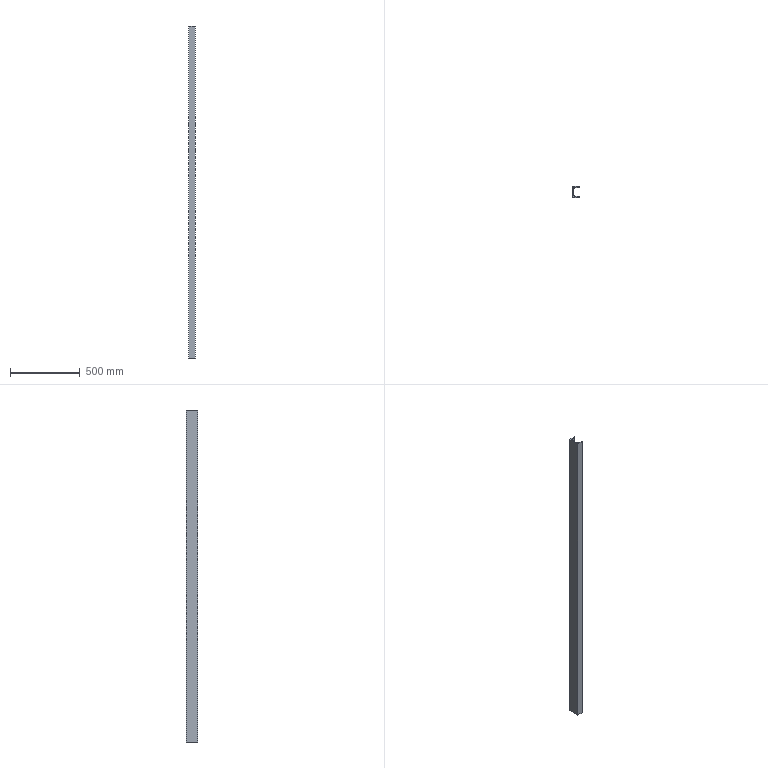Part | STEP file | 750038140 | 1 solid | 14 faces | box 43 x 80 x 2374 mm | volume 2431604 mm3 | plane 10 | cylinder 4 | commonest cylinder face diameters 8 x2 16 x2
STEP:
#1=CARTESIAN_POINT('',(0.,0.,2374.));
#2=VERTEX_POINT('',#1);
#3=CARTESIAN_POINT('',(0.,0.,0.));
#4=VERTEX_POINT('',#3);
#5=CARTESIAN_POINT('',(0.,0.,2374.));
#6=DIRECTION('',(0.,0.,-1.));
#7=VECTOR('',#6,1000.);
#8=LINE('',#5,#7);
#9=EDGE_CURVE('',#2,#4,#8,.T.);
#10=ORIENTED_EDGE('',*,*,#9,.F.);
#11=CARTESIAN_POINT('',(0.,80.,2374.));
#12=VERTEX_POINT('',#11);
#13=CARTESIAN_POINT('',(0.,80.,2374.));
#14=DIRECTION('',(0.,-1.,0.));
#15=VECTOR('',#14,1000.);
#16=LINE('',#13,#15);
#17=EDGE_CURVE('',#12,#2,#16,.T.);
#18=ORIENTED_EDGE('',*,*,#17,.F.);
#19=CARTESIAN_POINT('',(0.,80.,0.));
#20=VERTEX_POINT('',#19);
#21=CARTESIAN_POINT('',(0.,80.,2374.));
#22=DIRECTION('',(0.,0.,1.));
#23=VECTOR('',#22,1000.);
#24=LINE('',#21,#23);
#25=EDGE_CURVE('',#20,#12,#24,.T.);
#26=ORIENTED_EDGE('',*,*,#25,.F.);
#27=CARTESIAN_POINT('',(0.,80.,0.));
#28=DIRECTION('',(0.,1.,0.));
#29=VECTOR('',#28,1000.);
#30=LINE('',#27,#29);
#31=EDGE_CURVE('',#4,#20,#30,.T.);
#32=ORIENTED_EDGE('',*,*,#31,.F.);
#33=EDGE_LOOP('',(#10,#18,#26,#32));
#34=FACE_OUTER_BOUND('',#33,.T.);
#35=CARTESIAN_POINT('',(0.,80.,2374.));
#36=DIRECTION('',(1.,0.,0.));
#37=DIRECTION('',(0.,0.,-1.));
#38=AXIS2_PLACEMENT_3D('',#35,#36,#37);
#39=PLANE('',#38);
#40=ADVANCED_FACE('',(#34),#39,.F.);
#41=CARTESIAN_POINT('',(43.,80.,0.));
#42=VERTEX_POINT('',#41);
#43=CARTESIAN_POINT('',(39.,80.,0.));
#44=DIRECTION('',(-1.,0.,0.));
#45=VECTOR('',#44,1000.);
#46=LINE('',#43,#45);
#47=EDGE_CURVE('',#42,#20,#46,.T.);
#48=ORIENTED_EDGE('',*,*,#47,.F.);
#49=CARTESIAN_POINT('',(43.,77.52,0.));
#50=VERTEX_POINT('',#49);
#51=CARTESIAN_POINT('',(43.,2.48,0.));
#52=DIRECTION('',(0.,1.,0.));
#53=VECTOR('',#52,1000.);
#54=LINE('',#51,#53);
#55=EDGE_CURVE('',#50,#42,#54,.T.);
#56=ORIENTED_EDGE('',*,*,#55,.F.);
#57=CARTESIAN_POINT('',(39.398,73.54,0.));
#58=VERTEX_POINT('',#57);
#59=CARTESIAN_POINT('',(39.,77.52,0.));
#60=DIRECTION('',(0.,0.,1.));
#61=DIRECTION('',(-1.,0.,0.));
#62=AXIS2_PLACEMENT_3D('',#59,#60,#61);
#63=CIRCLE('',#62,4.);
#64=EDGE_CURVE('',#58,#50,#63,.T.);
#65=ORIENTED_EDGE('',*,*,#64,.F.);
#66=CARTESIAN_POINT('',(12.204,70.82,0.));
#67=VERTEX_POINT('',#66);
#68=CARTESIAN_POINT('',(12.204,70.82,0.));
#69=DIRECTION('',(0.995,0.0995,0.));
#70=VECTOR('',#69,1000.);
#71=LINE('',#68,#70);
#72=EDGE_CURVE('',#67,#58,#71,.T.);
#73=ORIENTED_EDGE('',*,*,#72,.F.);
#74=CARTESIAN_POINT('',(5.,62.86,0.));
#75=VERTEX_POINT('',#74);
#76=CARTESIAN_POINT('',(13.,62.86,0.));
#77=DIRECTION('',(0.,0.,-1.));
#78=DIRECTION('',(-1.,0.,0.));
#79=AXIS2_PLACEMENT_3D('',#76,#77,#78);
#80=CIRCLE('',#79,8.);
#81=EDGE_CURVE('',#75,#67,#80,.T.);
#82=ORIENTED_EDGE('',*,*,#81,.F.);
#83=CARTESIAN_POINT('',(5.,17.14,0.));
#84=VERTEX_POINT('',#83);
#85=CARTESIAN_POINT('',(5.,2.48,0.));
#86=DIRECTION('',(0.,1.,0.));
#87=VECTOR('',#86,1000.);
#88=LINE('',#85,#87);
#89=EDGE_CURVE('',#84,#75,#88,.T.);
#90=ORIENTED_EDGE('',*,*,#89,.F.);
#91=CARTESIAN_POINT('',(12.204,9.18,0.));
#92=VERTEX_POINT('',#91);
#93=CARTESIAN_POINT('',(13.,17.14,0.));
#94=DIRECTION('',(0.,0.,-1.));
#95=DIRECTION('',(-1.,0.,0.));
#96=AXIS2_PLACEMENT_3D('',#93,#94,#95);
#97=CIRCLE('',#96,8.);
#98=EDGE_CURVE('',#92,#84,#97,.T.);
#99=ORIENTED_EDGE('',*,*,#98,.F.);
#100=CARTESIAN_POINT('',(39.398,6.46,0.));
#101=VERTEX_POINT('',#100);
#102=CARTESIAN_POINT('',(39.398,6.46,0.));
#103=DIRECTION('',(-0.995,0.0995,0.));
#104=VECTOR('',#103,1000.);
#105=LINE('',#102,#104);
#106=EDGE_CURVE('',#101,#92,#105,.T.);
#107=ORIENTED_EDGE('',*,*,#106,.F.);
#108=CARTESIAN_POINT('',(43.,2.48,0.));
#109=VERTEX_POINT('',#108);
#110=CARTESIAN_POINT('',(39.,2.48,0.));
#111=DIRECTION('',(0.,0.,1.));
#112=DIRECTION('',(-1.,0.,0.));
#113=AXIS2_PLACEMENT_3D('',#110,#111,#112);
#114=CIRCLE('',#113,4.);
#115=EDGE_CURVE('',#109,#101,#114,.T.);
#116=ORIENTED_EDGE('',*,*,#115,.F.);
#117=CARTESIAN_POINT('',(43.,0.,0.));
#118=VERTEX_POINT('',#117);
#119=CARTESIAN_POINT('',(43.,2.48,0.));
#120=DIRECTION('',(0.,1.,0.));
#121=VECTOR('',#120,1000.);
#122=LINE('',#119,#121);
#123=EDGE_CURVE('',#118,#109,#122,.T.);
#124=ORIENTED_EDGE('',*,*,#123,.F.);
#125=CARTESIAN_POINT('',(39.,0.,0.));
#126=DIRECTION('',(1.,0.,0.));
#127=VECTOR('',#126,1000.);
#128=LINE('',#125,#127);
#129=EDGE_CURVE('',#4,#118,#128,.T.);
#130=ORIENTED_EDGE('',*,*,#129,.F.);
#131=ORIENTED_EDGE('',*,*,#31,.T.);
#132=EDGE_LOOP('',(#48,#56,#65,#73,#82,#90,#99,#107,#116,#124,#130,#131));
#133=FACE_OUTER_BOUND('',#132,.T.);
#134=CARTESIAN_POINT('',(39.,2.48,0.));
#135=DIRECTION('',(0.,0.,1.));
#136=DIRECTION('',(1.,0.,0.));
#137=AXIS2_PLACEMENT_3D('',#134,#135,#136);
#138=PLANE('',#137);
#139=ADVANCED_FACE('',(#133),#138,.F.);
#140=CARTESIAN_POINT('',(43.,0.,2374.));
#141=VERTEX_POINT('',#140);
#142=CARTESIAN_POINT('',(43.,0.,2374.));
#143=DIRECTION('',(0.,0.,-1.));
#144=VECTOR('',#143,1000.);
#145=LINE('',#142,#144);
#146=EDGE_CURVE('',#141,#118,#145,.T.);
#147=ORIENTED_EDGE('',*,*,#146,.F.);
#148=CARTESIAN_POINT('',(0.,0.,2374.));
#149=DIRECTION('',(1.,0.,0.));
#150=VECTOR('',#149,1000.);
#151=LINE('',#148,#150);
#152=EDGE_CURVE('',#2,#141,#151,.T.);
#153=ORIENTED_EDGE('',*,*,#152,.F.);
#154=ORIENTED_EDGE('',*,*,#9,.T.);
#155=ORIENTED_EDGE('',*,*,#129,.T.);
#156=EDGE_LOOP('',(#147,#153,#154,#155));
#157=FACE_OUTER_BOUND('',#156,.T.);
#158=CARTESIAN_POINT('',(0.,0.,2374.));
#159=DIRECTION('',(0.,1.,0.));
#160=DIRECTION('',(0.,0.,1.));
#161=AXIS2_PLACEMENT_3D('',#158,#159,#160);
#162=PLANE('',#161);
#163=ADVANCED_FACE('',(#157),#162,.F.);
#164=CARTESIAN_POINT('',(43.,77.52,2374.));
#165=VERTEX_POINT('',#164);
#166=CARTESIAN_POINT('',(43.,80.,2374.));
#167=VERTEX_POINT('',#166);
#168=CARTESIAN_POINT('',(43.,2.48,2374.));
#169=DIRECTION('',(0.,1.,0.));
#170=VECTOR('',#169,1000.);
#171=LINE('',#168,#170);
#172=EDGE_CURVE('',#165,#167,#171,.T.);
#173=ORIENTED_EDGE('',*,*,#172,.T.);
#174=CARTESIAN_POINT('',(39.,80.,2374.));
#175=DIRECTION('',(-1.,0.,0.));
#176=VECTOR('',#175,1000.);
#177=LINE('',#174,#176);
#178=EDGE_CURVE('',#167,#12,#177,.T.);
#179=ORIENTED_EDGE('',*,*,#178,.T.);
#180=ORIENTED_EDGE('',*,*,#17,.T.);
#181=ORIENTED_EDGE('',*,*,#152,.T.);
#182=CARTESIAN_POINT('',(43.,2.48,2374.));
#183=VERTEX_POINT('',#182);
#184=CARTESIAN_POINT('',(43.,2.48,2374.));
#185=DIRECTION('',(0.,1.,0.));
#186=VECTOR('',#185,1000.);
#187=LINE('',#184,#186);
#188=EDGE_CURVE('',#141,#183,#187,.T.);
#189=ORIENTED_EDGE('',*,*,#188,.T.);
#190=CARTESIAN_POINT('',(39.398,6.46,2374.));
#191=VERTEX_POINT('',#190);
#192=CARTESIAN_POINT('',(39.,2.48,2374.));
#193=DIRECTION('',(0.,0.,1.));
#194=DIRECTION('',(-1.,0.,0.));
#195=AXIS2_PLACEMENT_3D('',#192,#193,#194);
#196=CIRCLE('',#195,4.);
#197=EDGE_CURVE('',#183,#191,#196,.T.);
#198=ORIENTED_EDGE('',*,*,#197,.T.);
#199=CARTESIAN_POINT('',(12.204,9.18,2374.));
#200=VERTEX_POINT('',#199);
#201=CARTESIAN_POINT('',(39.398,6.46,2374.));
#202=DIRECTION('',(-0.995,0.0995,0.));
#203=VECTOR('',#202,1000.);
#204=LINE('',#201,#203);
#205=EDGE_CURVE('',#191,#200,#204,.T.);
#206=ORIENTED_EDGE('',*,*,#205,.T.);
#207=CARTESIAN_POINT('',(5.,17.14,2374.));
#208=VERTEX_POINT('',#207);
#209=CARTESIAN_POINT('',(13.,17.14,2374.));
#210=DIRECTION('',(0.,0.,-1.));
#211=DIRECTION('',(-1.,0.,0.));
#212=AXIS2_PLACEMENT_3D('',#209,#210,#211);
#213=CIRCLE('',#212,8.);
#214=EDGE_CURVE('',#200,#208,#213,.T.);
#215=ORIENTED_EDGE('',*,*,#214,.T.);
#216=CARTESIAN_POINT('',(5.,62.86,2374.));
#217=VERTEX_POINT('',#216);
#218=CARTESIAN_POINT('',(5.,2.48,2374.));
#219=DIRECTION('',(0.,1.,0.));
#220=VECTOR('',#219,1000.);
#221=LINE('',#218,#220);
#222=EDGE_CURVE('',#208,#217,#221,.T.);
#223=ORIENTED_EDGE('',*,*,#222,.T.);
#224=CARTESIAN_POINT('',(12.204,70.82,2374.));
#225=VERTEX_POINT('',#224);
#226=CARTESIAN_POINT('',(13.,62.86,2374.));
#227=DIRECTION('',(0.,0.,-1.));
#228=DIRECTION('',(-1.,0.,0.));
#229=AXIS2_PLACEMENT_3D('',#226,#227,#228);
#230=CIRCLE('',#229,8.);
#231=EDGE_CURVE('',#217,#225,#230,.T.);
#232=ORIENTED_EDGE('',*,*,#231,.T.);
#233=CARTESIAN_POINT('',(39.398,73.54,2374.));
#234=VERTEX_POINT('',#233);
#235=CARTESIAN_POINT('',(12.204,70.82,2374.));
#236=DIRECTION('',(0.995,0.0995,0.));
#237=VECTOR('',#236,1000.);
#238=LINE('',#235,#237);
#239=EDGE_CURVE('',#225,#234,#238,.T.);
#240=ORIENTED_EDGE('',*,*,#239,.T.);
#241=CARTESIAN_POINT('',(39.,77.52,2374.));
#242=DIRECTION('',(0.,0.,1.));
#243=DIRECTION('',(-1.,0.,0.));
#244=AXIS2_PLACEMENT_3D('',#241,#242,#243);
#245=CIRCLE('',#244,4.);
#246=EDGE_CURVE('',#234,#165,#245,.T.);
#247=ORIENTED_EDGE('',*,*,#246,.T.);
#248=EDGE_LOOP('',(#173,#179,#180,#181,#189,#198,#206,#215,#223,#232,#240,#247));
#249=FACE_OUTER_BOUND('',#248,.T.);
#250=CARTESIAN_POINT('',(39.,2.48,2374.));
#251=DIRECTION('',(0.,0.,1.));
#252=DIRECTION('',(1.,0.,0.));
#253=AXIS2_PLACEMENT_3D('',#250,#251,#252);
#254=PLANE('',#253);
#255=ADVANCED_FACE('',(#249),#254,.T.);
#256=ORIENTED_EDGE('',*,*,#25,.T.);
#257=ORIENTED_EDGE('',*,*,#178,.F.);
#258=CARTESIAN_POINT('',(43.,80.,2374.));
#259=DIRECTION('',(0.,0.,1.));
#260=VECTOR('',#259,1000.);
#261=LINE('',#258,#260);
#262=EDGE_CURVE('',#42,#167,#261,.T.);
#263=ORIENTED_EDGE('',*,*,#262,.F.);
#264=ORIENTED_EDGE('',*,*,#47,.T.);
#265=EDGE_LOOP('',(#256,#257,#263,#264));
#266=FACE_OUTER_BOUND('',#265,.T.);
#267=CARTESIAN_POINT('',(43.,80.,2374.));
#268=DIRECTION('',(0.,-1.,0.));
#269=DIRECTION('',(0.,0.,-1.));
#270=AXIS2_PLACEMENT_3D('',#267,#268,#269);
#271=PLANE('',#270);
#272=ADVANCED_FACE('',(#266),#271,.F.);
#273=ORIENTED_EDGE('',*,*,#262,.T.);
#274=ORIENTED_EDGE('',*,*,#172,.F.);
#275=CARTESIAN_POINT('',(43.,77.52,2374.));
#276=DIRECTION('',(0.,0.,1.));
#277=VECTOR('',#276,1000.);
#278=LINE('',#275,#277);
#279=EDGE_CURVE('',#50,#165,#278,.T.);
#280=ORIENTED_EDGE('',*,*,#279,.F.);
#281=ORIENTED_EDGE('',*,*,#55,.T.);
#282=EDGE_LOOP('',(#273,#274,#280,#281));
#283=FACE_OUTER_BOUND('',#282,.T.);
#284=CARTESIAN_POINT('',(43.,77.52,2374.));
#285=DIRECTION('',(-1.,0.,0.));
#286=DIRECTION('',(0.,0.,1.));
#287=AXIS2_PLACEMENT_3D('',#284,#285,#286);
#288=PLANE('',#287);
#289=ADVANCED_FACE('',(#283),#288,.F.);
#290=ORIENTED_EDGE('',*,*,#246,.F.);
#291=CARTESIAN_POINT('',(39.398,73.54,2374.));
#292=DIRECTION('',(0.,0.,-1.));
#293=VECTOR('',#292,1000.);
#294=LINE('',#291,#293);
#295=EDGE_CURVE('',#234,#58,#294,.T.);
#296=ORIENTED_EDGE('',*,*,#295,.T.);
#297=ORIENTED_EDGE('',*,*,#64,.T.);
#298=ORIENTED_EDGE('',*,*,#279,.T.);
#299=EDGE_LOOP('',(#290,#296,#297,#298));
#300=FACE_OUTER_BOUND('',#299,.T.);
#301=CARTESIAN_POINT('',(39.,77.52,2374.));
#302=DIRECTION('',(0.,0.,-1.));
#303=DIRECTION('',(-1.,0.,0.));
#304=AXIS2_PLACEMENT_3D('',#301,#302,#303);
#305=CYLINDRICAL_SURFACE('',#304,4.);
#306=ADVANCED_FACE('',(#300),#305,.T.);
#307=ORIENTED_EDGE('',*,*,#295,.F.);
#308=ORIENTED_EDGE('',*,*,#239,.F.);
#309=CARTESIAN_POINT('',(12.204,70.82,2374.));
#310=DIRECTION('',(0.,0.,1.));
#311=VECTOR('',#310,1000.);
#312=LINE('',#309,#311);
#313=EDGE_CURVE('',#67,#225,#312,.T.);
#314=ORIENTED_EDGE('',*,*,#313,.F.);
#315=ORIENTED_EDGE('',*,*,#72,.T.);
#316=EDGE_LOOP('',(#307,#308,#314,#315));
#317=FACE_OUTER_BOUND('',#316,.T.);
#318=CARTESIAN_POINT('',(12.204,70.82,2374.));
#319=DIRECTION('',(-0.0995,0.995,0.));
#320=DIRECTION('',(-0.995,-0.0995,0.));
#321=AXIS2_PLACEMENT_3D('',#318,#319,#320);
#322=PLANE('',#321);
#323=ADVANCED_FACE('',(#317),#322,.F.);
#324=ORIENTED_EDGE('',*,*,#313,.T.);
#325=ORIENTED_EDGE('',*,*,#231,.F.);
#326=CARTESIAN_POINT('',(5.,62.86,2374.));
#327=DIRECTION('',(0.,0.,1.));
#328=VECTOR('',#327,1000.);
#329=LINE('',#326,#328);
#330=EDGE_CURVE('',#75,#217,#329,.T.);
#331=ORIENTED_EDGE('',*,*,#330,.F.);
#332=ORIENTED_EDGE('',*,*,#81,.T.);
#333=EDGE_LOOP('',(#324,#325,#331,#332));
#334=FACE_OUTER_BOUND('',#333,.T.);
#335=CARTESIAN_POINT('',(13.,62.86,2374.));
#336=DIRECTION('',(0.,0.,-1.));
#337=DIRECTION('',(-1.,0.,0.));
#338=AXIS2_PLACEMENT_3D('',#335,#336,#337);
#339=CYLINDRICAL_SURFACE('',#338,8.);
#340=ADVANCED_FACE('',(#334),#339,.F.);
#341=ORIENTED_EDGE('',*,*,#330,.T.);
#342=ORIENTED_EDGE('',*,*,#222,.F.);
#343=CARTESIAN_POINT('',(5.,17.14,2374.));
#344=DIRECTION('',(0.,0.,1.));
#345=VECTOR('',#344,1000.);
#346=LINE('',#343,#345);
#347=EDGE_CURVE('',#84,#208,#346,.T.);
#348=ORIENTED_EDGE('',*,*,#347,.F.);
#349=ORIENTED_EDGE('',*,*,#89,.T.);
#350=EDGE_LOOP('',(#341,#342,#348,#349));
#351=FACE_OUTER_BOUND('',#350,.T.);
#352=CARTESIAN_POINT('',(5.,17.14,2374.));
#353=DIRECTION('',(-1.,0.,0.));
#354=DIRECTION('',(0.,-1.,0.));
#355=AXIS2_PLACEMENT_3D('',#352,#353,#354);
#356=PLANE('',#355);
#357=ADVANCED_FACE('',(#351),#356,.F.);
#358=ORIENTED_EDGE('',*,*,#347,.T.);
#359=ORIENTED_EDGE('',*,*,#214,.F.);
#360=CARTESIAN_POINT('',(12.204,9.18,2374.));
#361=DIRECTION('',(0.,0.,1.));
#362=VECTOR('',#361,1000.);
#363=LINE('',#360,#362);
#364=EDGE_CURVE('',#92,#200,#363,.T.);
#365=ORIENTED_EDGE('',*,*,#364,.F.);
#366=ORIENTED_EDGE('',*,*,#98,.T.);
#367=EDGE_LOOP('',(#358,#359,#365,#366));
#368=FACE_OUTER_BOUND('',#367,.T.);
#369=CARTESIAN_POINT('',(13.,17.14,2374.));
#370=DIRECTION('',(0.,0.,-1.));
#371=DIRECTION('',(-1.,0.,0.));
#372=AXIS2_PLACEMENT_3D('',#369,#370,#371);
#373=CYLINDRICAL_SURFACE('',#372,8.);
#374=ADVANCED_FACE('',(#368),#373,.F.);
#375=ORIENTED_EDGE('',*,*,#364,.T.);
#376=ORIENTED_EDGE('',*,*,#205,.F.);
#377=CARTESIAN_POINT('',(39.398,6.46,2374.));
#378=DIRECTION('',(0.,0.,1.));
#379=VECTOR('',#378,1000.);
#380=LINE('',#377,#379);
#381=EDGE_CURVE('',#101,#191,#380,.T.);
#382=ORIENTED_EDGE('',*,*,#381,.F.);
#383=ORIENTED_EDGE('',*,*,#106,.T.);
#384=EDGE_LOOP('',(#375,#376,#382,#383));
#385=FACE_OUTER_BOUND('',#384,.T.);
#386=CARTESIAN_POINT('',(39.398,6.46,2374.));
#387=DIRECTION('',(-0.0995,-0.995,0.));
#388=DIRECTION('',(0.995,-0.0995,0.));
#389=AXIS2_PLACEMENT_3D('',#386,#387,#388);
#390=PLANE('',#389);
#391=ADVANCED_FACE('',(#385),#390,.F.);
#392=ORIENTED_EDGE('',*,*,#197,.F.);
#393=CARTESIAN_POINT('',(43.,2.48,2374.));
#394=DIRECTION('',(0.,0.,-1.));
#395=VECTOR('',#394,1000.);
#396=LINE('',#393,#395);
#397=EDGE_CURVE('',#183,#109,#396,.T.);
#398=ORIENTED_EDGE('',*,*,#397,.T.);
#399=ORIENTED_EDGE('',*,*,#115,.T.);
#400=ORIENTED_EDGE('',*,*,#381,.T.);
#401=EDGE_LOOP('',(#392,#398,#399,#400));
#402=FACE_OUTER_BOUND('',#401,.T.);
#403=CARTESIAN_POINT('',(39.,2.48,2374.));
#404=DIRECTION('',(0.,0.,-1.));
#405=DIRECTION('',(-1.,0.,0.));
#406=AXIS2_PLACEMENT_3D('',#403,#404,#405);
#407=CYLINDRICAL_SURFACE('',#406,4.);
#408=ADVANCED_FACE('',(#402),#407,.T.);
#409=ORIENTED_EDGE('',*,*,#397,.F.);
#410=ORIENTED_EDGE('',*,*,#188,.F.);
#411=ORIENTED_EDGE('',*,*,#146,.T.);
#412=ORIENTED_EDGE('',*,*,#123,.T.);
#413=EDGE_LOOP('',(#409,#410,#411,#412));
#414=FACE_OUTER_BOUND('',#413,.T.);
#415=CARTESIAN_POINT('',(43.,0.,2374.));
#416=DIRECTION('',(-1.,0.,0.));
#417=DIRECTION('',(0.,0.,1.));
#418=AXIS2_PLACEMENT_3D('',#415,#416,#417);
#419=PLANE('',#418);
#420=ADVANCED_FACE('',(#414),#419,.F.);
#421=CLOSED_SHELL('',(#40,#139,#163,#255,#272,#289,#306,#323,#340,#357,#374,#391,#408,#420));
#422=MANIFOLD_SOLID_BREP('',#421);
#423=CARTESIAN_POINT('',(0.,0.,0.));
#424=DIRECTION('',(0.,0.,1.));
#425=DIRECTION('',(1.,0.,0.));
#426=AXIS2_PLACEMENT_3D('',#423,#424,#425);
#427=(LENGTH_UNIT()NAMED_UNIT(*)SI_UNIT(.MILLI.,.METRE.));
#428=UNCERTAINTY_MEASURE_WITH_UNIT(LENGTH_MEASURE(0.00001),#427,'','');
#429=(NAMED_UNIT(*)PLANE_ANGLE_UNIT()SI_UNIT($,.RADIAN.));
#430=(NAMED_UNIT(*)SI_UNIT($,.STERADIAN.)SOLID_ANGLE_UNIT());
#431=(GEOMETRIC_REPRESENTATION_CONTEXT(3)GLOBAL_UNCERTAINTY_ASSIGNED_CONTEXT((#428))GLOBAL_UNIT_ASSIGNED_CONTEXT((#427,#429,#430))REPRESENTATION_CONTEXT('',''));
#432=ADVANCED_BREP_SHAPE_REPRESENTATION('',(#422,#426),#431);